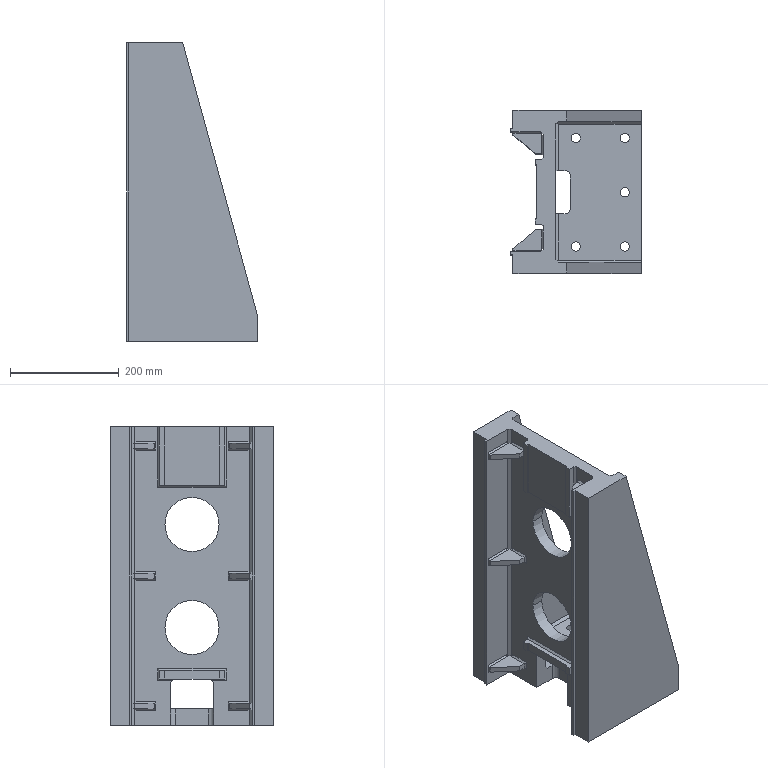Part | Creo | features CURVE 9, PROTRUSION 8, CUT 6, DATUM PLANE 3, CHAMFER 2, MOVE 2, COORDINATE SYSTEM 1, MIRROR 1, ROUND 1 | 1 solid | 140 faces | box 240.512 x 299.995 x 550 mm | volume 9242753 mm3 | plane 122 | cylinder 18 | commonest cylinder face diameters 17 x10 20 x4 100 x4